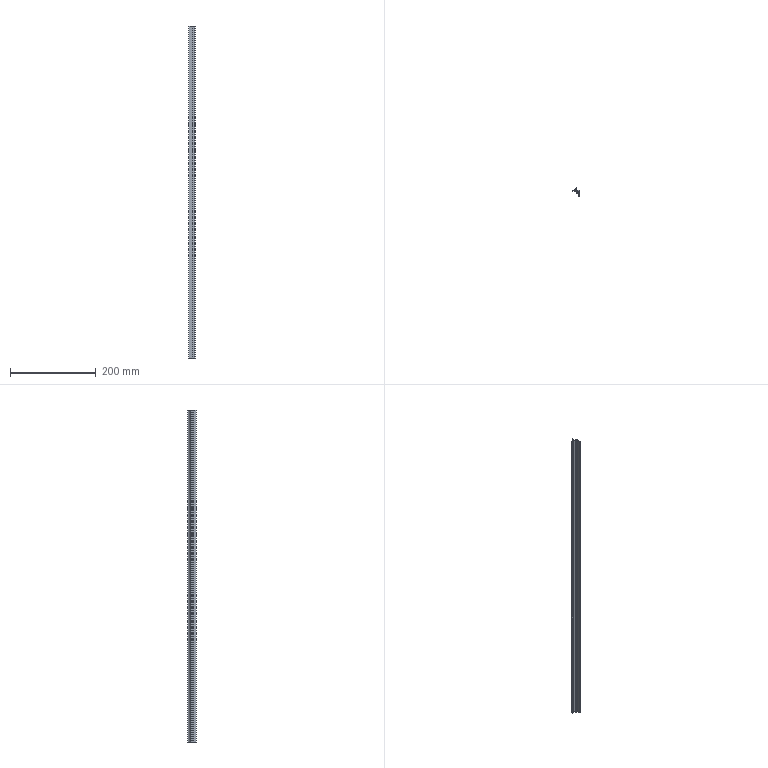Part | SolidWorks | features BaseBody 1, ICE 1, MoveFace 1 | 1 solid | 27 faces | box 14 x 20.3 x 774 mm | volume 39409 mm3 | plane 20 | cylinder 7 | commonest cylinder face diameters 0.387 x2 0.8 x2 0.4 x1 20 x1 22 x1
STEP:
#1=CARTESIAN_POINT('',(-5.304,-0.625,200.));
#2=VERTEX_POINT('',#1);
#3=CARTESIAN_POINT('',(-5.449,-0.8125,200.));
#4=VERTEX_POINT('',#3);
#5=CARTESIAN_POINT('',(-5.255,-0.8125,200.));
#6=DIRECTION('',(0.,0.,1.));
#7=DIRECTION('',(-1.,0.,0.));
#8=AXIS2_PLACEMENT_3D('',#5,#6,#7);
#9=CIRCLE('',#8,0.1937);
#10=EDGE_CURVE('',#2,#4,#9,.T.);
#11=ORIENTED_EDGE('',*,*,#10,.T.);
#12=CARTESIAN_POINT('',(-5.449,-0.8125,-574.));
#13=VERTEX_POINT('',#12);
#14=CARTESIAN_POINT('',(-5.449,-0.8125,230.));
#15=DIRECTION('',(0.,0.,-1.));
#16=VECTOR('',#15,1000.);
#17=LINE('',#14,#16);
#18=EDGE_CURVE('',#4,#13,#17,.T.);
#19=ORIENTED_EDGE('',*,*,#18,.T.);
#20=CARTESIAN_POINT('',(-5.304,-0.625,-574.));
#21=VERTEX_POINT('',#20);
#22=CARTESIAN_POINT('',(-5.255,-0.8125,-574.));
#23=DIRECTION('',(0.,0.,-1.));
#24=DIRECTION('',(1.,0.,0.));
#25=AXIS2_PLACEMENT_3D('',#22,#23,#24);
#26=CIRCLE('',#25,0.1937);
#27=EDGE_CURVE('',#13,#21,#26,.T.);
#28=ORIENTED_EDGE('',*,*,#27,.T.);
#29=CARTESIAN_POINT('',(-5.304,-0.625,230.));
#30=DIRECTION('',(0.,0.,-1.));
#31=VECTOR('',#30,1000.);
#32=LINE('',#29,#31);
#33=EDGE_CURVE('',#2,#21,#32,.T.);
#34=ORIENTED_EDGE('',*,*,#33,.F.);
#35=EDGE_LOOP('',(#11,#19,#28,#34));
#36=FACE_OUTER_BOUND('',#35,.T.);
#37=CARTESIAN_POINT('',(-5.255,-0.8125,230.));
#38=DIRECTION('',(0.,0.,-1.));
#39=DIRECTION('',(-1.,0.,0.));
#40=AXIS2_PLACEMENT_3D('',#37,#38,#39);
#41=CYLINDRICAL_SURFACE('',#40,0.1937);
#42=ADVANCED_FACE('',(#36),#41,.F.);
#43=CARTESIAN_POINT('',(5.,-1.,-574.));
#44=VERTEX_POINT('',#43);
#45=CARTESIAN_POINT('',(5.,-14.3,-574.));
#46=VERTEX_POINT('',#45);
#47=CARTESIAN_POINT('',(5.,29.623,-574.));
#48=DIRECTION('',(0.,-1.,0.));
#49=VECTOR('',#48,1000.);
#50=LINE('',#47,#49);
#51=EDGE_CURVE('',#44,#46,#50,.T.);
#52=ORIENTED_EDGE('',*,*,#51,.F.);
#53=CARTESIAN_POINT('',(5.,-1.,200.));
#54=VERTEX_POINT('',#53);
#55=CARTESIAN_POINT('',(5.,-1.,230.));
#56=DIRECTION('',(0.,0.,-1.));
#57=VECTOR('',#56,1000.);
#58=LINE('',#55,#57);
#59=EDGE_CURVE('',#54,#44,#58,.T.);
#60=ORIENTED_EDGE('',*,*,#59,.F.);
#61=CARTESIAN_POINT('',(5.,-14.3,200.));
#62=VERTEX_POINT('',#61);
#63=CARTESIAN_POINT('',(5.,-14.3,200.));
#64=DIRECTION('',(0.,1.,0.));
#65=VECTOR('',#64,1000.);
#66=LINE('',#63,#65);
#67=EDGE_CURVE('',#62,#54,#66,.T.);
#68=ORIENTED_EDGE('',*,*,#67,.F.);
#69=CARTESIAN_POINT('',(5.,-14.3,230.));
#70=DIRECTION('',(0.,0.,1.));
#71=VECTOR('',#70,1000.);
#72=LINE('',#69,#71);
#73=EDGE_CURVE('',#46,#62,#72,.T.);
#74=ORIENTED_EDGE('',*,*,#73,.F.);
#75=EDGE_LOOP('',(#52,#60,#68,#74));
#76=FACE_OUTER_BOUND('',#75,.T.);
#77=CARTESIAN_POINT('',(5.,-14.3,230.));
#78=DIRECTION('',(-1.,0.,0.));
#79=DIRECTION('',(0.,0.,1.));
#80=AXIS2_PLACEMENT_3D('',#77,#78,#79);
#81=PLANE('',#80);
#82=ADVANCED_FACE('',(#76),#81,.F.);
#83=CARTESIAN_POINT('',(-9.,-2.,-574.));
#84=VERTEX_POINT('',#83);
#85=CARTESIAN_POINT('',(-9.,-2.,200.));
#86=VERTEX_POINT('',#85);
#87=CARTESIAN_POINT('',(-9.,-2.,230.));
#88=DIRECTION('',(0.,0.,1.));
#89=VECTOR('',#88,1000.);
#90=LINE('',#87,#89);
#91=EDGE_CURVE('',#84,#86,#90,.T.);
#92=ORIENTED_EDGE('',*,*,#91,.F.);
#93=CARTESIAN_POINT('',(0.9,-2.,-574.));
#94=VERTEX_POINT('',#93);
#95=CARTESIAN_POINT('',(5.,-2.,-574.));
#96=DIRECTION('',(-1.,0.,0.));
#97=VECTOR('',#96,1000.);
#98=LINE('',#95,#97);
#99=EDGE_CURVE('',#94,#84,#98,.T.);
#100=ORIENTED_EDGE('',*,*,#99,.F.);
#101=CARTESIAN_POINT('',(0.9,-2.,200.));
#102=VERTEX_POINT('',#101);
#103=CARTESIAN_POINT('',(0.9,-2.,230.));
#104=DIRECTION('',(0.,0.,-1.));
#105=VECTOR('',#104,1000.);
#106=LINE('',#103,#105);
#107=EDGE_CURVE('',#102,#94,#106,.T.);
#108=ORIENTED_EDGE('',*,*,#107,.F.);
#109=CARTESIAN_POINT('',(5.,-2.,200.));
#110=DIRECTION('',(1.,0.,0.));
#111=VECTOR('',#110,1000.);
#112=LINE('',#109,#111);
#113=EDGE_CURVE('',#86,#102,#112,.T.);
#114=ORIENTED_EDGE('',*,*,#113,.F.);
#115=EDGE_LOOP('',(#92,#100,#108,#114));
#116=FACE_OUTER_BOUND('',#115,.T.);
#117=CARTESIAN_POINT('',(-9.,-2.,230.));
#118=DIRECTION('',(0.,1.,0.));
#119=DIRECTION('',(0.,0.,1.));
#120=AXIS2_PLACEMENT_3D('',#117,#118,#119);
#121=PLANE('',#120);
#122=ADVANCED_FACE('',(#116),#121,.F.);
#123=CARTESIAN_POINT('',(4.,-6.,200.));
#124=VERTEX_POINT('',#123);
#125=CARTESIAN_POINT('',(4.,-3.,200.));
#126=VERTEX_POINT('',#125);
#127=CARTESIAN_POINT('',(4.,29.623,200.));
#128=DIRECTION('',(0.,1.,0.));
#129=VECTOR('',#128,1000.);
#130=LINE('',#127,#129);
#131=EDGE_CURVE('',#124,#126,#130,.T.);
#132=ORIENTED_EDGE('',*,*,#131,.F.);
#133=CARTESIAN_POINT('',(1.,-6.,200.));
#134=VERTEX_POINT('',#133);
#135=CARTESIAN_POINT('',(5.,-6.,200.));
#136=DIRECTION('',(1.,0.,0.));
#137=VECTOR('',#136,1000.);
#138=LINE('',#135,#137);
#139=EDGE_CURVE('',#134,#124,#138,.T.);
#140=ORIENTED_EDGE('',*,*,#139,.F.);
#141=CARTESIAN_POINT('',(1.,-6.7,200.));
#142=VERTEX_POINT('',#141);
#143=CARTESIAN_POINT('',(1.,-6.,200.));
#144=DIRECTION('',(0.,-1.,0.));
#145=VECTOR('',#144,1000.);
#146=LINE('',#143,#145);
#147=EDGE_CURVE('',#134,#142,#146,.T.);
#148=ORIENTED_EDGE('',*,*,#147,.T.);
#149=CARTESIAN_POINT('',(-1.7,-6.7,200.));
#150=VERTEX_POINT('',#149);
#151=CARTESIAN_POINT('',(5.,-6.7,200.));
#152=DIRECTION('',(1.,0.,0.));
#153=VECTOR('',#152,1000.);
#154=LINE('',#151,#153);
#155=EDGE_CURVE('',#150,#142,#154,.T.);
#156=ORIENTED_EDGE('',*,*,#155,.F.);
#157=CARTESIAN_POINT('',(-1.7,-7.7,200.));
#158=VERTEX_POINT('',#157);
#159=CARTESIAN_POINT('',(-1.7,-6.7,200.));
#160=DIRECTION('',(0.,-1.,0.));
#161=VECTOR('',#160,1000.);
#162=LINE('',#159,#161);
#163=EDGE_CURVE('',#150,#158,#162,.T.);
#164=ORIENTED_EDGE('',*,*,#163,.T.);
#165=CARTESIAN_POINT('',(4.,-7.7,200.));
#166=VERTEX_POINT('',#165);
#167=CARTESIAN_POINT('',(5.,-7.7,200.));
#168=DIRECTION('',(-1.,0.,0.));
#169=VECTOR('',#168,1000.);
#170=LINE('',#167,#169);
#171=EDGE_CURVE('',#166,#158,#170,.T.);
#172=ORIENTED_EDGE('',*,*,#171,.F.);
#173=CARTESIAN_POINT('',(4.,-14.3,200.));
#174=VERTEX_POINT('',#173);
#175=CARTESIAN_POINT('',(4.,29.623,200.));
#176=DIRECTION('',(0.,1.,0.));
#177=VECTOR('',#176,1000.);
#178=LINE('',#175,#177);
#179=EDGE_CURVE('',#174,#166,#178,.T.);
#180=ORIENTED_EDGE('',*,*,#179,.F.);
#181=CARTESIAN_POINT('',(5.,-14.3,200.));
#182=DIRECTION('',(-1.,0.,0.));
#183=VECTOR('',#182,1000.);
#184=LINE('',#181,#183);
#185=EDGE_CURVE('',#62,#174,#184,.T.);
#186=ORIENTED_EDGE('',*,*,#185,.F.);
#187=ORIENTED_EDGE('',*,*,#67,.T.);
#188=CARTESIAN_POINT('',(-5.207,-1.,200.));
#189=VERTEX_POINT('',#188);
#190=CARTESIAN_POINT('',(5.,-1.,200.));
#191=DIRECTION('',(1.,0.,0.));
#192=VECTOR('',#191,1000.);
#193=LINE('',#190,#192);
#194=EDGE_CURVE('',#189,#54,#193,.T.);
#195=ORIENTED_EDGE('',*,*,#194,.F.);
#196=CARTESIAN_POINT('',(-5.255,-0.8125,200.));
#197=DIRECTION('',(0.,0.,1.));
#198=DIRECTION('',(-1.,0.,0.));
#199=AXIS2_PLACEMENT_3D('',#196,#197,#198);
#200=CIRCLE('',#199,0.1937);
#201=EDGE_CURVE('',#4,#189,#200,.T.);
#202=ORIENTED_EDGE('',*,*,#201,.F.);
#203=ORIENTED_EDGE('',*,*,#10,.F.);
#204=CARTESIAN_POINT('',(-1.368,3.063,200.));
#205=VERTEX_POINT('',#204);
#206=CARTESIAN_POINT('',(-10.628,9.,200.));
#207=DIRECTION('',(0.,0.,1.));
#208=DIRECTION('',(-1.,0.,0.));
#209=AXIS2_PLACEMENT_3D('',#206,#207,#208);
#210=CIRCLE('',#209,11.);
#211=EDGE_CURVE('',#2,#205,#210,.T.);
#212=ORIENTED_EDGE('',*,*,#211,.T.);
#213=CARTESIAN_POINT('',(-1.,2.955,200.));
#214=VERTEX_POINT('',#213);
#215=CARTESIAN_POINT('',(-1.2,2.955,200.));
#216=DIRECTION('',(0.,0.,1.));
#217=DIRECTION('',(-1.,0.,0.));
#218=AXIS2_PLACEMENT_3D('',#215,#216,#217);
#219=CIRCLE('',#218,0.2);
#220=EDGE_CURVE('',#214,#205,#219,.T.);
#221=ORIENTED_EDGE('',*,*,#220,.F.);
#222=CARTESIAN_POINT('',(-1.,1.5,200.));
#223=VERTEX_POINT('',#222);
#224=CARTESIAN_POINT('',(-1.,2.955,200.));
#225=DIRECTION('',(0.,1.,0.));
#226=VECTOR('',#225,1000.);
#227=LINE('',#224,#226);
#228=EDGE_CURVE('',#223,#214,#227,.T.);
#229=ORIENTED_EDGE('',*,*,#228,.F.);
#230=CARTESIAN_POINT('',(0.,1.5,200.));
#231=VERTEX_POINT('',#230);
#232=CARTESIAN_POINT('',(-1.,1.5,200.));
#233=DIRECTION('',(-1.,0.,0.));
#234=VECTOR('',#233,1000.);
#235=LINE('',#232,#234);
#236=EDGE_CURVE('',#231,#223,#235,.T.);
#237=ORIENTED_EDGE('',*,*,#236,.F.);
#238=CARTESIAN_POINT('',(0.,6.,200.));
#239=VERTEX_POINT('',#238);
#240=CARTESIAN_POINT('',(0.,1.5,200.));
#241=DIRECTION('',(0.,-1.,0.));
#242=VECTOR('',#241,1000.);
#243=LINE('',#240,#242);
#244=EDGE_CURVE('',#239,#231,#243,.T.);
#245=ORIENTED_EDGE('',*,*,#244,.F.);
#246=CARTESIAN_POINT('',(-0.8,6.,200.));
#247=VERTEX_POINT('',#246);
#248=CARTESIAN_POINT('',(0.,6.,200.));
#249=DIRECTION('',(1.,0.,0.));
#250=VECTOR('',#249,1000.);
#251=LINE('',#248,#250);
#252=EDGE_CURVE('',#247,#239,#251,.T.);
#253=ORIENTED_EDGE('',*,*,#252,.F.);
#254=CARTESIAN_POINT('',(-1.178,5.731,200.));
#255=VERTEX_POINT('',#254);
#256=CARTESIAN_POINT('',(-0.8,5.6,200.));
#257=DIRECTION('',(0.,0.,1.));
#258=DIRECTION('',(-1.,0.,0.));
#259=AXIS2_PLACEMENT_3D('',#256,#257,#258);
#260=CIRCLE('',#259,0.4);
#261=EDGE_CURVE('',#247,#255,#260,.T.);
#262=ORIENTED_EDGE('',*,*,#261,.T.);
#263=CARTESIAN_POINT('',(-8.678,-0.8077,200.));
#264=VERTEX_POINT('',#263);
#265=CARTESIAN_POINT('',(-10.628,9.,200.));
#266=DIRECTION('',(0.,0.,1.));
#267=DIRECTION('',(-1.,0.,0.));
#268=AXIS2_PLACEMENT_3D('',#265,#266,#267);
#269=CIRCLE('',#268,10.);
#270=EDGE_CURVE('',#264,#255,#269,.T.);
#271=ORIENTED_EDGE('',*,*,#270,.F.);
#272=CARTESIAN_POINT('',(-9.,-1.2,200.));
#273=VERTEX_POINT('',#272);
#274=CARTESIAN_POINT('',(-8.6,-1.2,200.));
#275=DIRECTION('',(0.,0.,1.));
#276=DIRECTION('',(-1.,0.,0.));
#277=AXIS2_PLACEMENT_3D('',#274,#275,#276);
#278=CIRCLE('',#277,0.4);
#279=EDGE_CURVE('',#264,#273,#278,.T.);
#280=ORIENTED_EDGE('',*,*,#279,.T.);
#281=CARTESIAN_POINT('',(-9.,8.,200.));
#282=DIRECTION('',(0.,-1.,0.));
#283=VECTOR('',#282,1000.);
#284=LINE('',#281,#283);
#285=EDGE_CURVE('',#273,#86,#284,.T.);
#286=ORIENTED_EDGE('',*,*,#285,.T.);
#287=ORIENTED_EDGE('',*,*,#113,.T.);
#288=CARTESIAN_POINT('',(0.9,-3.,200.));
#289=VERTEX_POINT('',#288);
#290=CARTESIAN_POINT('',(0.9,29.623,200.));
#291=DIRECTION('',(0.,1.,0.));
#292=VECTOR('',#291,1000.);
#293=LINE('',#290,#292);
#294=EDGE_CURVE('',#289,#102,#293,.T.);
#295=ORIENTED_EDGE('',*,*,#294,.F.);
#296=CARTESIAN_POINT('',(5.,-3.,200.));
#297=DIRECTION('',(-1.,0.,0.));
#298=VECTOR('',#297,1000.);
#299=LINE('',#296,#298);
#300=EDGE_CURVE('',#126,#289,#299,.T.);
#301=ORIENTED_EDGE('',*,*,#300,.F.);
#302=EDGE_LOOP('',(#132,#140,#148,#156,#164,#172,#180,#186,#187,#195,#202,#203,#212,#221,#229,#237,#245,#253,#262,#271,#280,#286,#287,#295,#301));
#303=FACE_OUTER_BOUND('',#302,.T.);
#304=CARTESIAN_POINT('',(5.,29.623,200.));
#305=DIRECTION('',(0.,0.,-1.));
#306=DIRECTION('',(-1.,0.,0.));
#307=AXIS2_PLACEMENT_3D('',#304,#305,#306);
#308=PLANE('',#307);
#309=ADVANCED_FACE('',(#303),#308,.F.);
#310=ORIENTED_EDGE('',*,*,#185,.T.);
#311=CARTESIAN_POINT('',(4.,-14.3,-574.));
#312=VERTEX_POINT('',#311);
#313=CARTESIAN_POINT('',(4.,-14.3,230.));
#314=DIRECTION('',(0.,0.,1.));
#315=VECTOR('',#314,1000.);
#316=LINE('',#313,#315);
#317=EDGE_CURVE('',#312,#174,#316,.T.);
#318=ORIENTED_EDGE('',*,*,#317,.F.);
#319=CARTESIAN_POINT('',(5.,-14.3,-574.));
#320=DIRECTION('',(-1.,0.,0.));
#321=VECTOR('',#320,1000.);
#322=LINE('',#319,#321);
#323=EDGE_CURVE('',#46,#312,#322,.T.);
#324=ORIENTED_EDGE('',*,*,#323,.F.);
#325=ORIENTED_EDGE('',*,*,#73,.T.);
#326=EDGE_LOOP('',(#310,#318,#324,#325));
#327=FACE_OUTER_BOUND('',#326,.T.);
#328=CARTESIAN_POINT('',(4.,-14.3,230.));
#329=DIRECTION('',(0.,1.,0.));
#330=DIRECTION('',(0.,0.,1.));
#331=AXIS2_PLACEMENT_3D('',#328,#329,#330);
#332=PLANE('',#331);
#333=ADVANCED_FACE('',(#327),#332,.F.);
#334=ORIENTED_EDGE('',*,*,#51,.T.);
#335=ORIENTED_EDGE('',*,*,#323,.T.);
#336=CARTESIAN_POINT('',(4.,-7.7,-574.));
#337=VERTEX_POINT('',#336);
#338=CARTESIAN_POINT('',(4.,-7.7,-574.));
#339=DIRECTION('',(0.,-1.,0.));
#340=VECTOR('',#339,1000.);
#341=LINE('',#338,#340);
#342=EDGE_CURVE('',#337,#312,#341,.T.);
#343=ORIENTED_EDGE('',*,*,#342,.F.);
#344=CARTESIAN_POINT('',(-1.7,-7.7,-574.));
#345=VERTEX_POINT('',#344);
#346=CARTESIAN_POINT('',(-1.7,-7.7,-574.));
#347=DIRECTION('',(1.,0.,0.));
#348=VECTOR('',#347,1000.);
#349=LINE('',#346,#348);
#350=EDGE_CURVE('',#345,#337,#349,.T.);
#351=ORIENTED_EDGE('',*,*,#350,.F.);
#352=CARTESIAN_POINT('',(-1.7,-6.7,-574.));
#353=VERTEX_POINT('',#352);
#354=CARTESIAN_POINT('',(-1.7,29.623,-574.));
#355=DIRECTION('',(0.,1.,0.));
#356=VECTOR('',#355,1000.);
#357=LINE('',#354,#356);
#358=EDGE_CURVE('',#345,#353,#357,.T.);
#359=ORIENTED_EDGE('',*,*,#358,.T.);
#360=CARTESIAN_POINT('',(1.,-6.7,-574.));
#361=VERTEX_POINT('',#360);
#362=CARTESIAN_POINT('',(1.,-6.7,-574.));
#363=DIRECTION('',(-1.,0.,0.));
#364=VECTOR('',#363,1000.);
#365=LINE('',#362,#364);
#366=EDGE_CURVE('',#361,#353,#365,.T.);
#367=ORIENTED_EDGE('',*,*,#366,.F.);
#368=CARTESIAN_POINT('',(1.,-6.,-574.));
#369=VERTEX_POINT('',#368);
#370=CARTESIAN_POINT('',(1.,29.623,-574.));
#371=DIRECTION('',(0.,1.,0.));
#372=VECTOR('',#371,1000.);
#373=LINE('',#370,#372);
#374=EDGE_CURVE('',#361,#369,#373,.T.);
#375=ORIENTED_EDGE('',*,*,#374,.T.);
#376=CARTESIAN_POINT('',(4.,-6.,-574.));
#377=VERTEX_POINT('',#376);
#378=CARTESIAN_POINT('',(4.,-6.,-574.));
#379=DIRECTION('',(-1.,0.,0.));
#380=VECTOR('',#379,1000.);
#381=LINE('',#378,#380);
#382=EDGE_CURVE('',#377,#369,#381,.T.);
#383=ORIENTED_EDGE('',*,*,#382,.F.);
#384=CARTESIAN_POINT('',(4.,-3.,-574.));
#385=VERTEX_POINT('',#384);
#386=CARTESIAN_POINT('',(4.,-3.,-574.));
#387=DIRECTION('',(0.,-1.,0.));
#388=VECTOR('',#387,1000.);
#389=LINE('',#386,#388);
#390=EDGE_CURVE('',#385,#377,#389,.T.);
#391=ORIENTED_EDGE('',*,*,#390,.F.);
#392=CARTESIAN_POINT('',(0.9,-3.,-574.));
#393=VERTEX_POINT('',#392);
#394=CARTESIAN_POINT('',(0.9,-3.,-574.));
#395=DIRECTION('',(1.,0.,0.));
#396=VECTOR('',#395,1000.);
#397=LINE('',#394,#396);
#398=EDGE_CURVE('',#393,#385,#397,.T.);
#399=ORIENTED_EDGE('',*,*,#398,.F.);
#400=CARTESIAN_POINT('',(0.9,-2.,-574.));
#401=DIRECTION('',(0.,-1.,0.));
#402=VECTOR('',#401,1000.);
#403=LINE('',#400,#402);
#404=EDGE_CURVE('',#94,#393,#403,.T.);
#405=ORIENTED_EDGE('',*,*,#404,.F.);
#406=ORIENTED_EDGE('',*,*,#99,.T.);
#407=CARTESIAN_POINT('',(-9.,-1.2,-574.));
#408=VERTEX_POINT('',#407);
#409=CARTESIAN_POINT('',(-9.,-1.2,-574.));
#410=DIRECTION('',(0.,-1.,0.));
#411=VECTOR('',#410,1000.);
#412=LINE('',#409,#411);
#413=EDGE_CURVE('',#408,#84,#412,.T.);
#414=ORIENTED_EDGE('',*,*,#413,.F.);
#415=CARTESIAN_POINT('',(-8.678,-0.8077,-574.));
#416=VERTEX_POINT('',#415);
#417=CARTESIAN_POINT('',(-8.6,-1.2,-574.));
#418=DIRECTION('',(0.,0.,-1.));
#419=DIRECTION('',(1.,0.,0.));
#420=AXIS2_PLACEMENT_3D('',#417,#418,#419);
#421=CIRCLE('',#420,0.4);
#422=EDGE_CURVE('',#408,#416,#421,.T.);
#423=ORIENTED_EDGE('',*,*,#422,.T.);
#424=CARTESIAN_POINT('',(-1.178,5.731,-574.));
#425=VERTEX_POINT('',#424);
#426=CARTESIAN_POINT('',(-10.628,9.,-574.));
#427=DIRECTION('',(0.,0.,-1.));
#428=DIRECTION('',(1.,0.,0.));
#429=AXIS2_PLACEMENT_3D('',#426,#427,#428);
#430=CIRCLE('',#429,10.);
#431=EDGE_CURVE('',#425,#416,#430,.T.);
#432=ORIENTED_EDGE('',*,*,#431,.F.);
#433=CARTESIAN_POINT('',(-0.8,6.,-574.));
#434=VERTEX_POINT('',#433);
#435=CARTESIAN_POINT('',(-0.8,5.6,-574.));
#436=DIRECTION('',(0.,0.,-1.));
#437=DIRECTION('',(1.,0.,0.));
#438=AXIS2_PLACEMENT_3D('',#435,#436,#437);
#439=CIRCLE('',#438,0.4);
#440=EDGE_CURVE('',#425,#434,#439,.T.);
#441=ORIENTED_EDGE('',*,*,#440,.T.);
#442=CARTESIAN_POINT('',(0.,6.,-574.));
#443=VERTEX_POINT('',#442);
#444=CARTESIAN_POINT('',(0.,6.,-574.));
#445=DIRECTION('',(-1.,0.,0.));
#446=VECTOR('',#445,1000.);
#447=LINE('',#444,#446);
#448=EDGE_CURVE('',#443,#434,#447,.T.);
#449=ORIENTED_EDGE('',*,*,#448,.F.);
#450=CARTESIAN_POINT('',(0.,1.5,-574.));
#451=VERTEX_POINT('',#450);
#452=CARTESIAN_POINT('',(0.,1.5,-574.));
#453=DIRECTION('',(0.,1.,0.));
#454=VECTOR('',#453,1000.);
#455=LINE('',#452,#454);
#456=EDGE_CURVE('',#451,#443,#455,.T.);
#457=ORIENTED_EDGE('',*,*,#456,.F.);
#458=CARTESIAN_POINT('',(-1.,1.5,-574.));
#459=VERTEX_POINT('',#458);
#460=CARTESIAN_POINT('',(-1.,1.5,-574.));
#461=DIRECTION('',(1.,0.,0.));
#462=VECTOR('',#461,1000.);
#463=LINE('',#460,#462);
#464=EDGE_CURVE('',#459,#451,#463,.T.);
#465=ORIENTED_EDGE('',*,*,#464,.F.);
#466=CARTESIAN_POINT('',(-1.,2.955,-574.));
#467=VERTEX_POINT('',#466);
#468=CARTESIAN_POINT('',(-1.,2.955,-574.));
#469=DIRECTION('',(0.,-1.,0.));
#470=VECTOR('',#469,1000.);
#471=LINE('',#468,#470);
#472=EDGE_CURVE('',#467,#459,#471,.T.);
#473=ORIENTED_EDGE('',*,*,#472,.F.);
#474=CARTESIAN_POINT('',(-1.368,3.063,-574.));
#475=VERTEX_POINT('',#474);
#476=CARTESIAN_POINT('',(-1.2,2.955,-574.));
#477=DIRECTION('',(0.,0.,-1.));
#478=DIRECTION('',(1.,0.,0.));
#479=AXIS2_PLACEMENT_3D('',#476,#477,#478);
#480=CIRCLE('',#479,0.2);
#481=EDGE_CURVE('',#475,#467,#480,.T.);
#482=ORIENTED_EDGE('',*,*,#481,.F.);
#483=CARTESIAN_POINT('',(-10.628,9.,-574.));
#484=DIRECTION('',(0.,0.,-1.));
#485=DIRECTION('',(1.,0.,0.));
#486=AXIS2_PLACEMENT_3D('',#483,#484,#485);
#487=CIRCLE('',#486,11.);
#488=EDGE_CURVE('',#475,#21,#487,.T.);
#489=ORIENTED_EDGE('',*,*,#488,.T.);
#490=ORIENTED_EDGE('',*,*,#27,.F.);
#491=CARTESIAN_POINT('',(-5.207,-1.,-574.));
#492=VERTEX_POINT('',#491);
#493=CARTESIAN_POINT('',(-5.255,-0.8125,-574.));
#494=DIRECTION('',(0.,0.,-1.));
#495=DIRECTION('',(1.,0.,0.));
#496=AXIS2_PLACEMENT_3D('',#493,#494,#495);
#497=CIRCLE('',#496,0.1937);
#498=EDGE_CURVE('',#492,#13,#497,.T.);
#499=ORIENTED_EDGE('',*,*,#498,.F.);
#500=CARTESIAN_POINT('',(5.,-1.,-574.));
#501=DIRECTION('',(-1.,0.,0.));
#502=VECTOR('',#501,1000.);
#503=LINE('',#500,#502);
#504=EDGE_CURVE('',#44,#492,#503,.T.);
#505=ORIENTED_EDGE('',*,*,#504,.F.);
#506=EDGE_LOOP('',(#334,#335,#343,#351,#359,#367,#375,#383,#391,#399,#405,#406,#414,#423,#432,#441,#449,#457,#465,#473,#482,#489,#490,#499,#505));
#507=FACE_OUTER_BOUND('',#506,.T.);
#508=CARTESIAN_POINT('',(5.,29.623,-574.));
#509=DIRECTION('',(0.,0.,1.));
#510=DIRECTION('',(1.,0.,0.));
#511=AXIS2_PLACEMENT_3D('',#508,#509,#510);
#512=PLANE('',#511);
#513=ADVANCED_FACE('',(#507),#512,.F.);
#514=ORIENTED_EDGE('',*,*,#59,.T.);
#515=ORIENTED_EDGE('',*,*,#504,.T.);
#516=CARTESIAN_POINT('',(-5.207,-1.,230.));
#517=DIRECTION('',(0.,0.,-1.));
#518=VECTOR('',#517,1000.);
#519=LINE('',#516,#518);
#520=EDGE_CURVE('',#189,#492,#519,.T.);
#521=ORIENTED_EDGE('',*,*,#520,.F.);
#522=ORIENTED_EDGE('',*,*,#194,.T.);
#523=EDGE_LOOP('',(#514,#515,#521,#522));
#524=FACE_OUTER_BOUND('',#523,.T.);
#525=CARTESIAN_POINT('',(5.,-1.,230.));
#526=DIRECTION('',(0.,-1.,0.));
#527=DIRECTION('',(0.,0.,-1.));
#528=AXIS2_PLACEMENT_3D('',#525,#526,#527);
#529=PLANE('',#528);
#530=ADVANCED_FACE('',(#524),#529,.F.);
#531=CARTESIAN_POINT('',(-9.,-1.2,230.));
#532=DIRECTION('',(0.,0.,1.));
#533=VECTOR('',#532,1000.);
#534=LINE('',#531,#533);
#535=EDGE_CURVE('',#408,#273,#534,.T.);
#536=ORIENTED_EDGE('',*,*,#535,.F.);
#537=ORIENTED_EDGE('',*,*,#413,.T.);
#538=ORIENTED_EDGE('',*,*,#91,.T.);
#539=ORIENTED_EDGE('',*,*,#285,.F.);
#540=EDGE_LOOP('',(#536,#537,#538,#539));
#541=FACE_OUTER_BOUND('',#540,.T.);
#542=CARTESIAN_POINT('',(-9.,-1.2,230.));
#543=DIRECTION('',(1.,0.,0.));
#544=DIRECTION('',(0.,0.,-1.));
#545=AXIS2_PLACEMENT_3D('',#542,#543,#544);
#546=PLANE('',#545);
#547=ADVANCED_FACE('',(#541),#546,.F.);
#548=ORIENTED_EDGE('',*,*,#294,.T.);
#549=ORIENTED_EDGE('',*,*,#107,.T.);
#550=ORIENTED_EDGE('',*,*,#404,.T.);
#551=CARTESIAN_POINT('',(0.9,-3.,230.));
#552=DIRECTION('',(0.,0.,-1.));
#553=VECTOR('',#552,1000.);
#554=LINE('',#551,#553);
#555=EDGE_CURVE('',#289,#393,#554,.T.);
#556=ORIENTED_EDGE('',*,*,#555,.F.);
#557=EDGE_LOOP('',(#548,#549,#550,#556));
#558=FACE_OUTER_BOUND('',#557,.T.);
#559=CARTESIAN_POINT('',(0.9,-2.,230.));
#560=DIRECTION('',(1.,0.,0.));
#561=DIRECTION('',(0.,0.,-1.));
#562=AXIS2_PLACEMENT_3D('',#559,#560,#561);
#563=PLANE('',#562);
#564=ADVANCED_FACE('',(#558),#563,.F.);
#565=ORIENTED_EDGE('',*,*,#300,.T.);
#566=ORIENTED_EDGE('',*,*,#555,.T.);
#567=ORIENTED_EDGE('',*,*,#398,.T.);
#568=CARTESIAN_POINT('',(4.,-3.,230.));
#569=DIRECTION('',(0.,0.,-1.));
#570=VECTOR('',#569,1000.);
#571=LINE('',#568,#570);
#572=EDGE_CURVE('',#126,#385,#571,.T.);
#573=ORIENTED_EDGE('',*,*,#572,.F.);
#574=EDGE_LOOP('',(#565,#566,#567,#573));
#575=FACE_OUTER_BOUND('',#574,.T.);
#576=CARTESIAN_POINT('',(0.9,-3.,230.));
#577=DIRECTION('',(0.,1.,0.));
#578=DIRECTION('',(0.,0.,1.));
#579=AXIS2_PLACEMENT_3D('',#576,#577,#578);
#580=PLANE('',#579);
#581=ADVANCED_FACE('',(#575),#580,.F.);
#582=ORIENTED_EDGE('',*,*,#131,.T.);
#583=ORIENTED_EDGE('',*,*,#572,.T.);
#584=ORIENTED_EDGE('',*,*,#390,.T.);
#585=CARTESIAN_POINT('',(4.,-6.,230.));
#586=DIRECTION('',(0.,0.,-1.));
#587=VECTOR('',#586,1000.);
#588=LINE('',#585,#587);
#589=EDGE_CURVE('',#124,#377,#588,.T.);
#590=ORIENTED_EDGE('',*,*,#589,.F.);
#591=EDGE_LOOP('',(#582,#583,#584,#590));
#592=FACE_OUTER_BOUND('',#591,.T.);
#593=CARTESIAN_POINT('',(4.,-3.,230.));
#594=DIRECTION('',(1.,0.,0.));
#595=DIRECTION('',(0.,0.,-1.));
#596=AXIS2_PLACEMENT_3D('',#593,#594,#595);
#597=PLANE('',#596);
#598=ADVANCED_FACE('',(#592),#597,.F.);
#599=ORIENTED_EDGE('',*,*,#139,.T.);
#600=ORIENTED_EDGE('',*,*,#589,.T.);
#601=ORIENTED_EDGE('',*,*,#382,.T.);
#602=CARTESIAN_POINT('',(1.,-6.,230.));
#603=DIRECTION('',(0.,0.,-1.));
#604=VECTOR('',#603,1000.);
#605=LINE('',#602,#604);
#606=EDGE_CURVE('',#134,#369,#605,.T.);
#607=ORIENTED_EDGE('',*,*,#606,.F.);
#608=EDGE_LOOP('',(#599,#600,#601,#607));
#609=FACE_OUTER_BOUND('',#608,.T.);
#610=CARTESIAN_POINT('',(4.,-6.,230.));
#611=DIRECTION('',(0.,-1.,0.));
#612=DIRECTION('',(0.,0.,-1.));
#613=AXIS2_PLACEMENT_3D('',#610,#611,#612);
#614=PLANE('',#613);
#615=ADVANCED_FACE('',(#609),#614,.F.);
#616=ORIENTED_EDGE('',*,*,#155,.T.);
#617=CARTESIAN_POINT('',(1.,-6.7,230.));
#618=DIRECTION('',(0.,0.,1.));
#619=VECTOR('',#618,1000.);
#620=LINE('',#617,#619);
#621=EDGE_CURVE('',#361,#142,#620,.T.);
#622=ORIENTED_EDGE('',*,*,#621,.F.);
#623=ORIENTED_EDGE('',*,*,#366,.T.);
#624=CARTESIAN_POINT('',(-1.7,-6.7,230.));
#625=DIRECTION('',(0.,0.,-1.));
#626=VECTOR('',#625,1000.);
#627=LINE('',#624,#626);
#628=EDGE_CURVE('',#150,#353,#627,.T.);
#629=ORIENTED_EDGE('',*,*,#628,.F.);
#630=EDGE_LOOP('',(#616,#622,#623,#629));
#631=FACE_OUTER_BOUND('',#630,.T.);
#632=CARTESIAN_POINT('',(1.,-6.7,230.));
#633=DIRECTION('',(0.,-1.,0.));
#634=DIRECTION('',(0.,0.,-1.));
#635=AXIS2_PLACEMENT_3D('',#632,#633,#634);
#636=PLANE('',#635);
#637=ADVANCED_FACE('',(#631),#636,.F.);
#638=ORIENTED_EDGE('',*,*,#171,.T.);
#639=CARTESIAN_POINT('',(-1.7,-7.7,230.));
#640=DIRECTION('',(0.,0.,1.));
#641=VECTOR('',#640,1000.);
#642=LINE('',#639,#641);
#643=EDGE_CURVE('',#345,#158,#642,.T.);
#644=ORIENTED_EDGE('',*,*,#643,.F.);
#645=ORIENTED_EDGE('',*,*,#350,.T.);
#646=CARTESIAN_POINT('',(4.,-7.7,230.));
#647=DIRECTION('',(0.,0.,-1.));
#648=VECTOR('',#647,1000.);
#649=LINE('',#646,#648);
#650=EDGE_CURVE('',#166,#337,#649,.T.);
#651=ORIENTED_EDGE('',*,*,#650,.F.);
#652=EDGE_LOOP('',(#638,#644,#645,#651));
#653=FACE_OUTER_BOUND('',#652,.T.);
#654=CARTESIAN_POINT('',(-1.7,-7.7,230.));
#655=DIRECTION('',(0.,1.,0.));
#656=DIRECTION('',(0.,0.,1.));
#657=AXIS2_PLACEMENT_3D('',#654,#655,#656);
#658=PLANE('',#657);
#659=ADVANCED_FACE('',(#653),#658,.F.);
#660=ORIENTED_EDGE('',*,*,#179,.T.);
#661=ORIENTED_EDGE('',*,*,#650,.T.);
#662=ORIENTED_EDGE('',*,*,#342,.T.);
#663=ORIENTED_EDGE('',*,*,#317,.T.);
#664=EDGE_LOOP('',(#660,#661,#662,#663));
#665=FACE_OUTER_BOUND('',#664,.T.);
#666=CARTESIAN_POINT('',(4.,-7.7,230.));
#667=DIRECTION('',(1.,0.,0.));
#668=DIRECTION('',(0.,0.,-1.));
#669=AXIS2_PLACEMENT_3D('',#666,#667,#668);
#670=PLANE('',#669);
#671=ADVANCED_FACE('',(#665),#670,.F.);
#672=ORIENTED_EDGE('',*,*,#18,.F.);
#673=ORIENTED_EDGE('',*,*,#201,.T.);
#674=ORIENTED_EDGE('',*,*,#520,.T.);
#675=ORIENTED_EDGE('',*,*,#498,.T.);
#676=EDGE_LOOP('',(#672,#673,#674,#675));
#677=FACE_OUTER_BOUND('',#676,.T.);
#678=CARTESIAN_POINT('',(-5.255,-0.8125,230.));
#679=DIRECTION('',(0.,0.,-1.));
#680=DIRECTION('',(-1.,0.,0.));
#681=AXIS2_PLACEMENT_3D('',#678,#679,#680);
#682=CYLINDRICAL_SURFACE('',#681,0.1937);
#683=ADVANCED_FACE('',(#677),#682,.F.);
#684=CARTESIAN_POINT('',(-1.,2.955,230.));
#685=DIRECTION('',(0.,0.,1.));
#686=VECTOR('',#685,1000.);
#687=LINE('',#684,#686);
#688=EDGE_CURVE('',#467,#214,#687,.T.);
#689=ORIENTED_EDGE('',*,*,#688,.F.);
#690=ORIENTED_EDGE('',*,*,#472,.T.);
#691=CARTESIAN_POINT('',(-1.,1.5,230.));
#692=DIRECTION('',(0.,0.,-1.));
#693=VECTOR('',#692,1000.);
#694=LINE('',#691,#693);
#695=EDGE_CURVE('',#223,#459,#694,.T.);
#696=ORIENTED_EDGE('',*,*,#695,.F.);
#697=ORIENTED_EDGE('',*,*,#228,.T.);
#698=EDGE_LOOP('',(#689,#690,#696,#697));
#699=FACE_OUTER_BOUND('',#698,.T.);
#700=CARTESIAN_POINT('',(-1.,2.955,230.));
#701=DIRECTION('',(1.,0.,0.));
#702=DIRECTION('',(0.,0.,-1.));
#703=AXIS2_PLACEMENT_3D('',#700,#701,#702);
#704=PLANE('',#703);
#705=ADVANCED_FACE('',(#699),#704,.F.);
#706=ORIENTED_EDGE('',*,*,#488,.F.);
#707=CARTESIAN_POINT('',(-1.368,3.063,230.));
#708=DIRECTION('',(0.,0.,1.));
#709=VECTOR('',#708,1000.);
#710=LINE('',#707,#709);
#711=EDGE_CURVE('',#475,#205,#710,.T.);
#712=ORIENTED_EDGE('',*,*,#711,.T.);
#713=ORIENTED_EDGE('',*,*,#211,.F.);
#714=ORIENTED_EDGE('',*,*,#33,.T.);
#715=EDGE_LOOP('',(#706,#712,#713,#714));
#716=FACE_OUTER_BOUND('',#715,.T.);
#717=CARTESIAN_POINT('',(-10.628,9.,230.));
#718=DIRECTION('',(0.,0.,-1.));
#719=DIRECTION('',(-1.,0.,0.));
#720=AXIS2_PLACEMENT_3D('',#717,#718,#719);
#721=CYLINDRICAL_SURFACE('',#720,11.);
#722=ADVANCED_FACE('',(#716),#721,.T.);
#723=CARTESIAN_POINT('',(-1.178,5.731,230.));
#724=DIRECTION('',(0.,0.,1.));
#725=VECTOR('',#724,1000.);
#726=LINE('',#723,#725);
#727=EDGE_CURVE('',#425,#255,#726,.T.);
#728=ORIENTED_EDGE('',*,*,#727,.F.);
#729=ORIENTED_EDGE('',*,*,#431,.T.);
#730=CARTESIAN_POINT('',(-8.678,-0.8077,230.));
#731=DIRECTION('',(0.,0.,-1.));
#732=VECTOR('',#731,1000.);
#733=LINE('',#730,#732);
#734=EDGE_CURVE('',#264,#416,#733,.T.);
#735=ORIENTED_EDGE('',*,*,#734,.F.);
#736=ORIENTED_EDGE('',*,*,#270,.T.);
#737=EDGE_LOOP('',(#728,#729,#735,#736));
#738=FACE_OUTER_BOUND('',#737,.T.);
#739=CARTESIAN_POINT('',(-10.628,9.,230.));
#740=DIRECTION('',(0.,0.,-1.));
#741=DIRECTION('',(-1.,0.,0.));
#742=AXIS2_PLACEMENT_3D('',#739,#740,#741);
#743=CYLINDRICAL_SURFACE('',#742,10.);
#744=ADVANCED_FACE('',(#738),#743,.F.);
#745=CARTESIAN_POINT('',(0.,1.5,230.));
#746=DIRECTION('',(0.,0.,1.));
#747=VECTOR('',#746,1000.);
#748=LINE('',#745,#747);
#749=EDGE_CURVE('',#451,#231,#748,.T.);
#750=ORIENTED_EDGE('',*,*,#749,.F.);
#751=ORIENTED_EDGE('',*,*,#456,.T.);
#752=CARTESIAN_POINT('',(0.,6.,230.));
#753=DIRECTION('',(0.,0.,-1.));
#754=VECTOR('',#753,1000.);
#755=LINE('',#752,#754);
#756=EDGE_CURVE('',#239,#443,#755,.T.);
#757=ORIENTED_EDGE('',*,*,#756,.F.);
#758=ORIENTED_EDGE('',*,*,#244,.T.);
#759=EDGE_LOOP('',(#750,#751,#757,#758));
#760=FACE_OUTER_BOUND('',#759,.T.);
#761=CARTESIAN_POINT('',(0.,1.5,230.));
#762=DIRECTION('',(-1.,0.,0.));
#763=DIRECTION('',(0.,0.,1.));
#764=AXIS2_PLACEMENT_3D('',#761,#762,#763);
#765=PLANE('',#764);
#766=ADVANCED_FACE('',(#760),#765,.F.);
#767=ORIENTED_EDGE('',*,*,#422,.F.);
#768=ORIENTED_EDGE('',*,*,#535,.T.);
#769=ORIENTED_EDGE('',*,*,#279,.F.);
#770=ORIENTED_EDGE('',*,*,#734,.T.);
#771=EDGE_LOOP('',(#767,#768,#769,#770));
#772=FACE_OUTER_BOUND('',#771,.T.);
#773=CARTESIAN_POINT('',(-8.6,-1.2,230.));
#774=DIRECTION('',(0.,0.,-1.));
#775=DIRECTION('',(-1.,0.,0.));
#776=AXIS2_PLACEMENT_3D('',#773,#774,#775);
#777=CYLINDRICAL_SURFACE('',#776,0.4);
#778=ADVANCED_FACE('',(#772),#777,.T.);
#779=ORIENTED_EDGE('',*,*,#147,.F.);
#780=ORIENTED_EDGE('',*,*,#606,.T.);
#781=ORIENTED_EDGE('',*,*,#374,.F.);
#782=ORIENTED_EDGE('',*,*,#621,.T.);
#783=EDGE_LOOP('',(#779,#780,#781,#782));
#784=FACE_OUTER_BOUND('',#783,.T.);
#785=CARTESIAN_POINT('',(1.,-6.,230.));
#786=DIRECTION('',(1.,0.,0.));
#787=DIRECTION('',(0.,0.,-1.));
#788=AXIS2_PLACEMENT_3D('',#785,#786,#787);
#789=PLANE('',#788);
#790=ADVANCED_FACE('',(#784),#789,.F.);
#791=ORIENTED_EDGE('',*,*,#163,.F.);
#792=ORIENTED_EDGE('',*,*,#628,.T.);
#793=ORIENTED_EDGE('',*,*,#358,.F.);
#794=ORIENTED_EDGE('',*,*,#643,.T.);
#795=EDGE_LOOP('',(#791,#792,#793,#794));
#796=FACE_OUTER_BOUND('',#795,.T.);
#797=CARTESIAN_POINT('',(-1.7,-6.7,230.));
#798=DIRECTION('',(1.,0.,0.));
#799=DIRECTION('',(0.,0.,-1.));
#800=AXIS2_PLACEMENT_3D('',#797,#798,#799);
#801=PLANE('',#800);
#802=ADVANCED_FACE('',(#796),#801,.F.);
#803=ORIENTED_EDGE('',*,*,#711,.F.);
#804=ORIENTED_EDGE('',*,*,#481,.T.);
#805=ORIENTED_EDGE('',*,*,#688,.T.);
#806=ORIENTED_EDGE('',*,*,#220,.T.);
#807=EDGE_LOOP('',(#803,#804,#805,#806));
#808=FACE_OUTER_BOUND('',#807,.T.);
#809=CARTESIAN_POINT('',(-1.2,2.955,230.));
#810=DIRECTION('',(0.,0.,-1.));
#811=DIRECTION('',(-1.,0.,0.));
#812=AXIS2_PLACEMENT_3D('',#809,#810,#811);
#813=CYLINDRICAL_SURFACE('',#812,0.2);
#814=ADVANCED_FACE('',(#808),#813,.F.);
#815=ORIENTED_EDGE('',*,*,#695,.T.);
#816=ORIENTED_EDGE('',*,*,#464,.T.);
#817=ORIENTED_EDGE('',*,*,#749,.T.);
#818=ORIENTED_EDGE('',*,*,#236,.T.);
#819=EDGE_LOOP('',(#815,#816,#817,#818));
#820=FACE_OUTER_BOUND('',#819,.T.);
#821=CARTESIAN_POINT('',(-1.,1.5,230.));
#822=DIRECTION('',(0.,1.,0.));
#823=DIRECTION('',(0.,0.,1.));
#824=AXIS2_PLACEMENT_3D('',#821,#822,#823);
#825=PLANE('',#824);
#826=ADVANCED_FACE('',(#820),#825,.F.);
#827=ORIENTED_EDGE('',*,*,#440,.F.);
#828=ORIENTED_EDGE('',*,*,#727,.T.);
#829=ORIENTED_EDGE('',*,*,#261,.F.);
#830=CARTESIAN_POINT('',(-0.8,6.,230.));
#831=DIRECTION('',(0.,0.,-1.));
#832=VECTOR('',#831,1000.);
#833=LINE('',#830,#832);
#834=EDGE_CURVE('',#247,#434,#833,.T.);
#835=ORIENTED_EDGE('',*,*,#834,.T.);
#836=EDGE_LOOP('',(#827,#828,#829,#835));
#837=FACE_OUTER_BOUND('',#836,.T.);
#838=CARTESIAN_POINT('',(-0.8,5.6,230.));
#839=DIRECTION('',(0.,0.,-1.));
#840=DIRECTION('',(-1.,0.,0.));
#841=AXIS2_PLACEMENT_3D('',#838,#839,#840);
#842=CYLINDRICAL_SURFACE('',#841,0.4);
#843=ADVANCED_FACE('',(#837),#842,.T.);
#844=ORIENTED_EDGE('',*,*,#756,.T.);
#845=ORIENTED_EDGE('',*,*,#448,.T.);
#846=ORIENTED_EDGE('',*,*,#834,.F.);
#847=ORIENTED_EDGE('',*,*,#252,.T.);
#848=EDGE_LOOP('',(#844,#845,#846,#847));
#849=FACE_OUTER_BOUND('',#848,.T.);
#850=CARTESIAN_POINT('',(0.,6.,230.));
#851=DIRECTION('',(0.,-1.,0.));
#852=DIRECTION('',(0.,0.,-1.));
#853=AXIS2_PLACEMENT_3D('',#850,#851,#852);
#854=PLANE('',#853);
#855=ADVANCED_FACE('',(#849),#854,.F.);
#856=CLOSED_SHELL('',(#42,#82,#122,#309,#333,#513,#530,#547,#564,#581,#598,#615,#637,#659,#671,#683,#705,#722,#744,#766,#778,#790,#802,#814,#826,#843,#855));
#857=MANIFOLD_SOLID_BREP('',#856);
#858=CARTESIAN_POINT('',(0.,0.,0.));
#859=DIRECTION('',(0.,0.,1.));
#860=DIRECTION('',(1.,0.,0.));
#861=AXIS2_PLACEMENT_3D('',#858,#859,#860);
#862=(LENGTH_UNIT()NAMED_UNIT(*)SI_UNIT(.MILLI.,.METRE.));
#863=UNCERTAINTY_MEASURE_WITH_UNIT(LENGTH_MEASURE(0.00001),#862,'','');
#864=(NAMED_UNIT(*)PLANE_ANGLE_UNIT()SI_UNIT($,.RADIAN.));
#865=(NAMED_UNIT(*)SI_UNIT($,.STERADIAN.)SOLID_ANGLE_UNIT());
#866=(GEOMETRIC_REPRESENTATION_CONTEXT(3)GLOBAL_UNCERTAINTY_ASSIGNED_CONTEXT((#863))GLOBAL_UNIT_ASSIGNED_CONTEXT((#862,#864,#865))REPRESENTATION_CONTEXT('',''));
#867=ADVANCED_BREP_SHAPE_REPRESENTATION('',(#857,#861),#866);